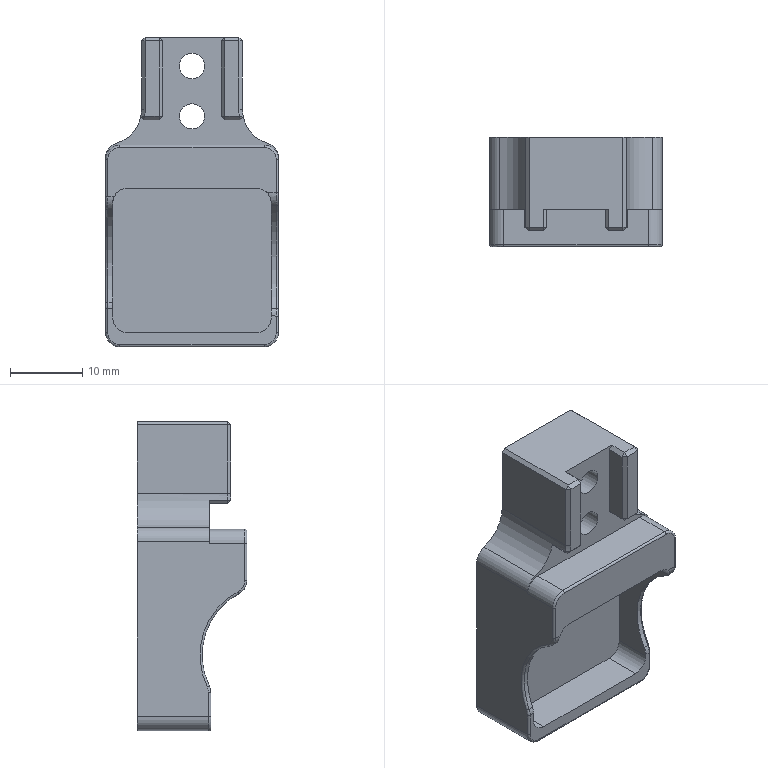Part | 1 solid | 84 faces | box 24 x 15.2 x 43 mm | volume 7498 mm3 | plane 46 | cylinder 20 | spline 8 | torus 6 | cone 4 | commonest cylinder face diameters 4 x10 0.6 x6 3.5 x2 10 x2